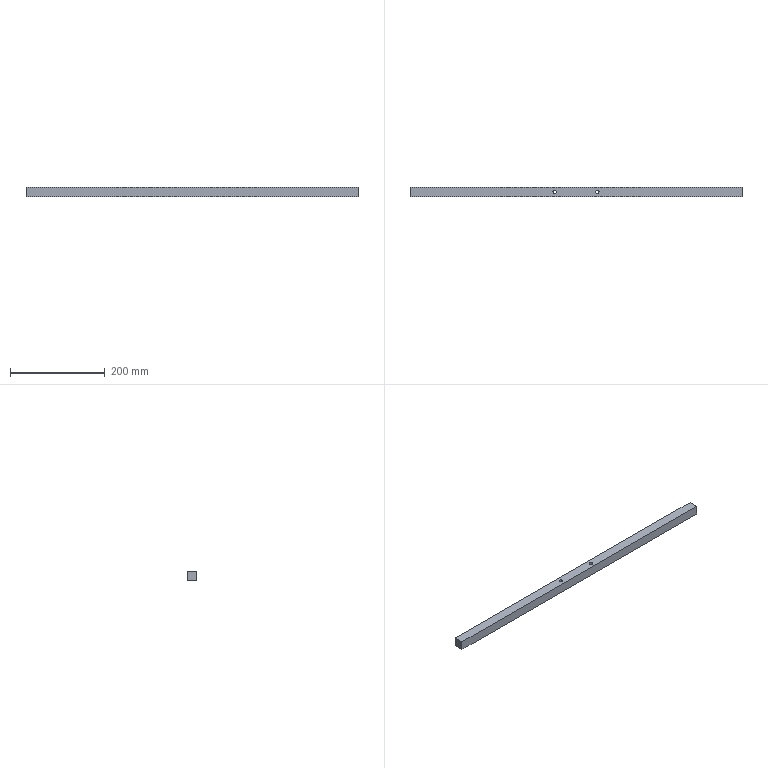Part | SolidWorks | features Extrusion 1, ICE 1 | 1 solid | 10 faces | box 700 x 20 x 20 mm | volume 278461 mm3 | plane 6 | cylinder 4 | commonest cylinder face diameters 7 x4
STEP:
#1=CARTESIAN_POINT('',(41.5,0.,-10.));
#2=VERTEX_POINT('',#1);
#3=CARTESIAN_POINT('',(48.5,0.,-10.));
#4=VERTEX_POINT('',#3);
#5=CARTESIAN_POINT('',(45.,0.,-10.));
#6=DIRECTION('',(0.,0.,1.));
#7=DIRECTION('',(1.,0.,0.));
#8=AXIS2_PLACEMENT_3D('',#5,#6,#7);
#9=CIRCLE('',#8,3.5);
#10=EDGE_CURVE('',#2,#4,#9,.T.);
#11=ORIENTED_EDGE('',*,*,#10,.F.);
#12=CARTESIAN_POINT('',(41.5,0.,10.));
#13=VERTEX_POINT('',#12);
#14=CARTESIAN_POINT('',(41.5,0.,-690.));
#15=DIRECTION('',(0.,0.,1.));
#16=VECTOR('',#15,1000.);
#17=LINE('',#14,#16);
#18=EDGE_CURVE('',#2,#13,#17,.T.);
#19=ORIENTED_EDGE('',*,*,#18,.T.);
#20=CARTESIAN_POINT('',(48.5,0.,10.));
#21=VERTEX_POINT('',#20);
#22=CARTESIAN_POINT('',(45.,0.,10.));
#23=DIRECTION('',(0.,0.,1.));
#24=DIRECTION('',(1.,0.,0.));
#25=AXIS2_PLACEMENT_3D('',#22,#23,#24);
#26=CIRCLE('',#25,3.5);
#27=EDGE_CURVE('',#13,#21,#26,.T.);
#28=ORIENTED_EDGE('',*,*,#27,.T.);
#29=CARTESIAN_POINT('',(48.5,0.,-690.));
#30=DIRECTION('',(0.,0.,1.));
#31=VECTOR('',#30,1000.);
#32=LINE('',#29,#31);
#33=EDGE_CURVE('',#4,#21,#32,.T.);
#34=ORIENTED_EDGE('',*,*,#33,.F.);
#35=EDGE_LOOP('',(#11,#19,#28,#34));
#36=FACE_OUTER_BOUND('',#35,.T.);
#37=CARTESIAN_POINT('',(45.,0.,-690.));
#38=DIRECTION('',(0.,0.,1.));
#39=DIRECTION('',(1.,0.,0.));
#40=AXIS2_PLACEMENT_3D('',#37,#38,#39);
#41=CYLINDRICAL_SURFACE('',#40,3.5);
#42=ADVANCED_FACE('',(#36),#41,.F.);
#43=CARTESIAN_POINT('',(-48.5,0.,-10.));
#44=VERTEX_POINT('',#43);
#45=CARTESIAN_POINT('',(-41.5,0.,-10.));
#46=VERTEX_POINT('',#45);
#47=CARTESIAN_POINT('',(-45.,0.,-10.));
#48=DIRECTION('',(0.,0.,1.));
#49=DIRECTION('',(1.,0.,0.));
#50=AXIS2_PLACEMENT_3D('',#47,#48,#49);
#51=CIRCLE('',#50,3.5);
#52=EDGE_CURVE('',#44,#46,#51,.T.);
#53=ORIENTED_EDGE('',*,*,#52,.F.);
#54=CARTESIAN_POINT('',(-48.5,0.,10.));
#55=VERTEX_POINT('',#54);
#56=CARTESIAN_POINT('',(-48.5,0.,-690.));
#57=DIRECTION('',(0.,0.,1.));
#58=VECTOR('',#57,1000.);
#59=LINE('',#56,#58);
#60=EDGE_CURVE('',#44,#55,#59,.T.);
#61=ORIENTED_EDGE('',*,*,#60,.T.);
#62=CARTESIAN_POINT('',(-41.5,0.,10.));
#63=VERTEX_POINT('',#62);
#64=CARTESIAN_POINT('',(-45.,0.,10.));
#65=DIRECTION('',(0.,0.,1.));
#66=DIRECTION('',(1.,0.,0.));
#67=AXIS2_PLACEMENT_3D('',#64,#65,#66);
#68=CIRCLE('',#67,3.5);
#69=EDGE_CURVE('',#55,#63,#68,.T.);
#70=ORIENTED_EDGE('',*,*,#69,.T.);
#71=CARTESIAN_POINT('',(-41.5,0.,-690.));
#72=DIRECTION('',(0.,0.,1.));
#73=VECTOR('',#72,1000.);
#74=LINE('',#71,#73);
#75=EDGE_CURVE('',#46,#63,#74,.T.);
#76=ORIENTED_EDGE('',*,*,#75,.F.);
#77=EDGE_LOOP('',(#53,#61,#70,#76));
#78=FACE_OUTER_BOUND('',#77,.T.);
#79=CARTESIAN_POINT('',(-45.,0.,-690.));
#80=DIRECTION('',(0.,0.,1.));
#81=DIRECTION('',(1.,0.,0.));
#82=AXIS2_PLACEMENT_3D('',#79,#80,#81);
#83=CYLINDRICAL_SURFACE('',#82,3.5);
#84=ADVANCED_FACE('',(#78),#83,.F.);
#85=CARTESIAN_POINT('',(45.,0.,-10.));
#86=DIRECTION('',(0.,0.,1.));
#87=DIRECTION('',(1.,0.,0.));
#88=AXIS2_PLACEMENT_3D('',#85,#86,#87);
#89=CIRCLE('',#88,3.5);
#90=EDGE_CURVE('',#4,#2,#89,.T.);
#91=ORIENTED_EDGE('',*,*,#90,.T.);
#92=ORIENTED_EDGE('',*,*,#10,.T.);
#93=EDGE_LOOP('',(#91,#92));
#94=FACE_BOUND('',#93,.T.);
#95=CARTESIAN_POINT('',(-45.,0.,-10.));
#96=DIRECTION('',(0.,0.,1.));
#97=DIRECTION('',(1.,0.,0.));
#98=AXIS2_PLACEMENT_3D('',#95,#96,#97);
#99=CIRCLE('',#98,3.5);
#100=EDGE_CURVE('',#46,#44,#99,.T.);
#101=ORIENTED_EDGE('',*,*,#100,.T.);
#102=ORIENTED_EDGE('',*,*,#52,.T.);
#103=EDGE_LOOP('',(#101,#102));
#104=FACE_BOUND('',#103,.T.);
#105=CARTESIAN_POINT('',(-350.,-10.,-10.));
#106=VERTEX_POINT('',#105);
#107=CARTESIAN_POINT('',(-350.,10.,-10.));
#108=VERTEX_POINT('',#107);
#109=CARTESIAN_POINT('',(-350.,10.,-10.));
#110=DIRECTION('',(0.,1.,0.));
#111=VECTOR('',#110,1000.);
#112=LINE('',#109,#111);
#113=EDGE_CURVE('',#106,#108,#112,.T.);
#114=ORIENTED_EDGE('',*,*,#113,.T.);
#115=CARTESIAN_POINT('',(350.,10.,-10.));
#116=VERTEX_POINT('',#115);
#117=CARTESIAN_POINT('',(350.,10.,-10.));
#118=DIRECTION('',(-1.,0.,0.));
#119=VECTOR('',#118,1000.);
#120=LINE('',#117,#119);
#121=EDGE_CURVE('',#116,#108,#120,.T.);
#122=ORIENTED_EDGE('',*,*,#121,.F.);
#123=CARTESIAN_POINT('',(350.,-10.,-10.));
#124=VERTEX_POINT('',#123);
#125=CARTESIAN_POINT('',(350.,10.,-10.));
#126=DIRECTION('',(0.,1.,0.));
#127=VECTOR('',#126,1000.);
#128=LINE('',#125,#127);
#129=EDGE_CURVE('',#124,#116,#128,.T.);
#130=ORIENTED_EDGE('',*,*,#129,.F.);
#131=CARTESIAN_POINT('',(350.,-10.,-10.));
#132=DIRECTION('',(-1.,0.,0.));
#133=VECTOR('',#132,1000.);
#134=LINE('',#131,#133);
#135=EDGE_CURVE('',#124,#106,#134,.T.);
#136=ORIENTED_EDGE('',*,*,#135,.T.);
#137=EDGE_LOOP('',(#114,#122,#130,#136));
#138=FACE_OUTER_BOUND('',#137,.T.);
#139=CARTESIAN_POINT('',(350.,10.,-10.));
#140=DIRECTION('',(0.,0.,1.));
#141=DIRECTION('',(1.,0.,0.));
#142=AXIS2_PLACEMENT_3D('',#139,#140,#141);
#143=PLANE('',#142);
#144=ADVANCED_FACE('',(#94,#104,#138),#143,.F.);
#145=CARTESIAN_POINT('',(-350.,10.,10.));
#146=VERTEX_POINT('',#145);
#147=CARTESIAN_POINT('',(-350.,10.,10.));
#148=DIRECTION('',(0.,0.,1.));
#149=VECTOR('',#148,1000.);
#150=LINE('',#147,#149);
#151=EDGE_CURVE('',#108,#146,#150,.T.);
#152=ORIENTED_EDGE('',*,*,#151,.T.);
#153=CARTESIAN_POINT('',(350.,10.,10.));
#154=VERTEX_POINT('',#153);
#155=CARTESIAN_POINT('',(350.,10.,10.));
#156=DIRECTION('',(-1.,0.,0.));
#157=VECTOR('',#156,1000.);
#158=LINE('',#155,#157);
#159=EDGE_CURVE('',#154,#146,#158,.T.);
#160=ORIENTED_EDGE('',*,*,#159,.F.);
#161=CARTESIAN_POINT('',(350.,10.,10.));
#162=DIRECTION('',(0.,0.,1.));
#163=VECTOR('',#162,1000.);
#164=LINE('',#161,#163);
#165=EDGE_CURVE('',#116,#154,#164,.T.);
#166=ORIENTED_EDGE('',*,*,#165,.F.);
#167=ORIENTED_EDGE('',*,*,#121,.T.);
#168=EDGE_LOOP('',(#152,#160,#166,#167));
#169=FACE_OUTER_BOUND('',#168,.T.);
#170=CARTESIAN_POINT('',(350.,10.,10.));
#171=DIRECTION('',(0.,-1.,0.));
#172=DIRECTION('',(0.,0.,-1.));
#173=AXIS2_PLACEMENT_3D('',#170,#171,#172);
#174=PLANE('',#173);
#175=ADVANCED_FACE('',(#169),#174,.F.);
#176=CARTESIAN_POINT('',(45.,0.,10.));
#177=DIRECTION('',(0.,0.,1.));
#178=DIRECTION('',(1.,0.,0.));
#179=AXIS2_PLACEMENT_3D('',#176,#177,#178);
#180=CIRCLE('',#179,3.5);
#181=EDGE_CURVE('',#21,#13,#180,.T.);
#182=ORIENTED_EDGE('',*,*,#181,.F.);
#183=ORIENTED_EDGE('',*,*,#27,.F.);
#184=EDGE_LOOP('',(#182,#183));
#185=FACE_BOUND('',#184,.T.);
#186=CARTESIAN_POINT('',(-45.,0.,10.));
#187=DIRECTION('',(0.,0.,1.));
#188=DIRECTION('',(1.,0.,0.));
#189=AXIS2_PLACEMENT_3D('',#186,#187,#188);
#190=CIRCLE('',#189,3.5);
#191=EDGE_CURVE('',#63,#55,#190,.T.);
#192=ORIENTED_EDGE('',*,*,#191,.F.);
#193=ORIENTED_EDGE('',*,*,#69,.F.);
#194=EDGE_LOOP('',(#192,#193));
#195=FACE_BOUND('',#194,.T.);
#196=CARTESIAN_POINT('',(-350.,-10.,10.));
#197=VERTEX_POINT('',#196);
#198=CARTESIAN_POINT('',(-350.,10.,10.));
#199=DIRECTION('',(0.,-1.,0.));
#200=VECTOR('',#199,1000.);
#201=LINE('',#198,#200);
#202=EDGE_CURVE('',#146,#197,#201,.T.);
#203=ORIENTED_EDGE('',*,*,#202,.T.);
#204=CARTESIAN_POINT('',(350.,-10.,10.));
#205=VERTEX_POINT('',#204);
#206=CARTESIAN_POINT('',(350.,-10.,10.));
#207=DIRECTION('',(-1.,0.,0.));
#208=VECTOR('',#207,1000.);
#209=LINE('',#206,#208);
#210=EDGE_CURVE('',#205,#197,#209,.T.);
#211=ORIENTED_EDGE('',*,*,#210,.F.);
#212=CARTESIAN_POINT('',(350.,10.,10.));
#213=DIRECTION('',(0.,-1.,0.));
#214=VECTOR('',#213,1000.);
#215=LINE('',#212,#214);
#216=EDGE_CURVE('',#154,#205,#215,.T.);
#217=ORIENTED_EDGE('',*,*,#216,.F.);
#218=ORIENTED_EDGE('',*,*,#159,.T.);
#219=EDGE_LOOP('',(#203,#211,#217,#218));
#220=FACE_OUTER_BOUND('',#219,.T.);
#221=CARTESIAN_POINT('',(350.,10.,10.));
#222=DIRECTION('',(0.,0.,-1.));
#223=DIRECTION('',(0.,1.,0.));
#224=AXIS2_PLACEMENT_3D('',#221,#222,#223);
#225=PLANE('',#224);
#226=ADVANCED_FACE('',(#185,#195,#220),#225,.F.);
#227=CARTESIAN_POINT('',(-350.,-10.,10.));
#228=DIRECTION('',(0.,0.,-1.));
#229=VECTOR('',#228,1000.);
#230=LINE('',#227,#229);
#231=EDGE_CURVE('',#197,#106,#230,.T.);
#232=ORIENTED_EDGE('',*,*,#231,.T.);
#233=ORIENTED_EDGE('',*,*,#135,.F.);
#234=CARTESIAN_POINT('',(350.,-10.,10.));
#235=DIRECTION('',(0.,0.,-1.));
#236=VECTOR('',#235,1000.);
#237=LINE('',#234,#236);
#238=EDGE_CURVE('',#205,#124,#237,.T.);
#239=ORIENTED_EDGE('',*,*,#238,.F.);
#240=ORIENTED_EDGE('',*,*,#210,.T.);
#241=EDGE_LOOP('',(#232,#233,#239,#240));
#242=FACE_OUTER_BOUND('',#241,.T.);
#243=CARTESIAN_POINT('',(350.,-10.,10.));
#244=DIRECTION('',(0.,1.,0.));
#245=DIRECTION('',(0.,0.,1.));
#246=AXIS2_PLACEMENT_3D('',#243,#244,#245);
#247=PLANE('',#246);
#248=ADVANCED_FACE('',(#242),#247,.F.);
#249=ORIENTED_EDGE('',*,*,#129,.T.);
#250=ORIENTED_EDGE('',*,*,#165,.T.);
#251=ORIENTED_EDGE('',*,*,#216,.T.);
#252=ORIENTED_EDGE('',*,*,#238,.T.);
#253=EDGE_LOOP('',(#249,#250,#251,#252));
#254=FACE_OUTER_BOUND('',#253,.T.);
#255=CARTESIAN_POINT('',(350.,0.,0.));
#256=DIRECTION('',(1.,0.,0.));
#257=DIRECTION('',(0.,0.,-1.));
#258=AXIS2_PLACEMENT_3D('',#255,#256,#257);
#259=PLANE('',#258);
#260=ADVANCED_FACE('',(#254),#259,.T.);
#261=ORIENTED_EDGE('',*,*,#113,.F.);
#262=ORIENTED_EDGE('',*,*,#231,.F.);
#263=ORIENTED_EDGE('',*,*,#202,.F.);
#264=ORIENTED_EDGE('',*,*,#151,.F.);
#265=EDGE_LOOP('',(#261,#262,#263,#264));
#266=FACE_OUTER_BOUND('',#265,.T.);
#267=CARTESIAN_POINT('',(-350.,0.,0.));
#268=DIRECTION('',(1.,0.,0.));
#269=DIRECTION('',(0.,0.,-1.));
#270=AXIS2_PLACEMENT_3D('',#267,#268,#269);
#271=PLANE('',#270);
#272=ADVANCED_FACE('',(#266),#271,.F.);
#273=ORIENTED_EDGE('',*,*,#60,.F.);
#274=ORIENTED_EDGE('',*,*,#100,.F.);
#275=ORIENTED_EDGE('',*,*,#75,.T.);
#276=ORIENTED_EDGE('',*,*,#191,.T.);
#277=EDGE_LOOP('',(#273,#274,#275,#276));
#278=FACE_OUTER_BOUND('',#277,.T.);
#279=CARTESIAN_POINT('',(-45.,0.,-690.));
#280=DIRECTION('',(0.,0.,1.));
#281=DIRECTION('',(1.,0.,0.));
#282=AXIS2_PLACEMENT_3D('',#279,#280,#281);
#283=CYLINDRICAL_SURFACE('',#282,3.5);
#284=ADVANCED_FACE('',(#278),#283,.F.);
#285=ORIENTED_EDGE('',*,*,#18,.F.);
#286=ORIENTED_EDGE('',*,*,#90,.F.);
#287=ORIENTED_EDGE('',*,*,#33,.T.);
#288=ORIENTED_EDGE('',*,*,#181,.T.);
#289=EDGE_LOOP('',(#285,#286,#287,#288));
#290=FACE_OUTER_BOUND('',#289,.T.);
#291=CARTESIAN_POINT('',(45.,0.,-690.));
#292=DIRECTION('',(0.,0.,1.));
#293=DIRECTION('',(1.,0.,0.));
#294=AXIS2_PLACEMENT_3D('',#291,#292,#293);
#295=CYLINDRICAL_SURFACE('',#294,3.5);
#296=ADVANCED_FACE('',(#290),#295,.F.);
#297=CLOSED_SHELL('',(#42,#84,#144,#175,#226,#248,#260,#272,#284,#296));
#298=MANIFOLD_SOLID_BREP('',#297);
#299=CARTESIAN_POINT('',(0.,0.,0.));
#300=DIRECTION('',(0.,0.,1.));
#301=DIRECTION('',(1.,0.,0.));
#302=AXIS2_PLACEMENT_3D('',#299,#300,#301);
#303=(LENGTH_UNIT()NAMED_UNIT(*)SI_UNIT(.MILLI.,.METRE.));
#304=UNCERTAINTY_MEASURE_WITH_UNIT(LENGTH_MEASURE(0.00001),#303,'','');
#305=(NAMED_UNIT(*)PLANE_ANGLE_UNIT()SI_UNIT($,.RADIAN.));
#306=(NAMED_UNIT(*)SI_UNIT($,.STERADIAN.)SOLID_ANGLE_UNIT());
#307=(GEOMETRIC_REPRESENTATION_CONTEXT(3)GLOBAL_UNCERTAINTY_ASSIGNED_CONTEXT((#304))GLOBAL_UNIT_ASSIGNED_CONTEXT((#303,#305,#306))REPRESENTATION_CONTEXT('',''));
#308=ADVANCED_BREP_SHAPE_REPRESENTATION('',(#298,#302),#307);